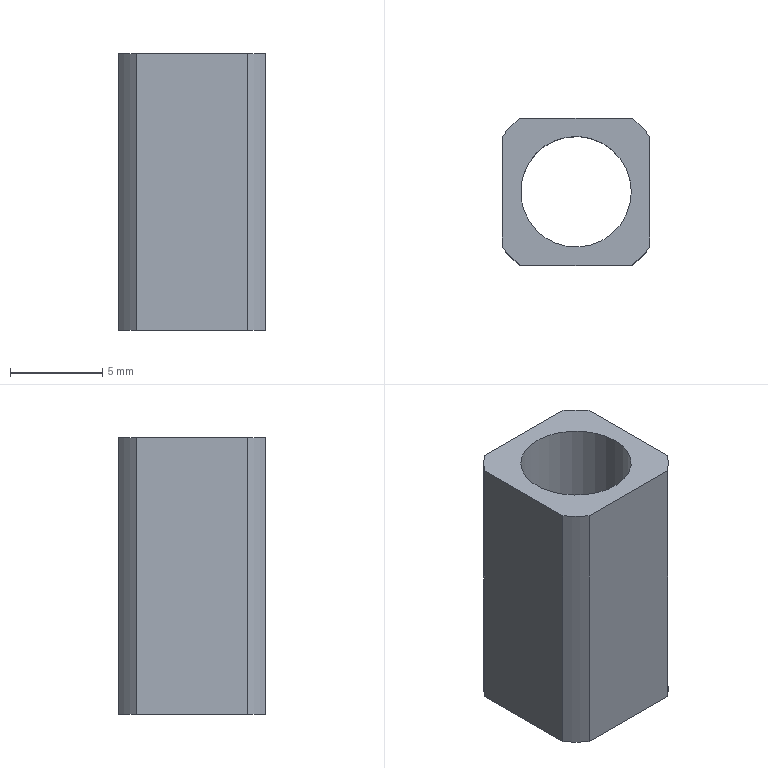NC program | NX | posted with a generic post | part box 8 x 8 x 15 mm
Whole program:
N10 G17 G21 G94 G90
(PLANAR_MILL , TOOL : D8开粗)
N12 T01 M6
N14 G53
N16 G17 G0 G90 X15.25 Y0. S2000 M3
N18 G43 Z10.05 H1
N20 Z2.05
N22 G94 G1 Z0.05 F800.
N24 X5.25
N26 G2 X0. Y-5.25 R5.25
N28 X5.25 Y0. R-5.25
N30 G1 X15.25
N32 Z2.05
N34 G0 Z10.05
(ADAPTIVE_MILLING , TOOL : D8开粗)
N36 Z10.15 S3000
N38 X-17.042 Y-1.094
N40 Z-13.
N42 G1 X-16.892 Y-1.097 Z-13.937 F1000.
N44 X-16.742 Y-1.099 Z-14.308
N46 X-16.592 Y-1.102 Z-14.58
N48 X-16.442 Y-1.105 Z-14.8
N50 X-16.292 Y-1.107 Z-14.984
N52 X-16.142 Y-1.11 Z-15.142
N54 X-15.992 Y-1.113 Z-15.28
N56 X-15.842 Y-1.115 Z-15.4
N58 X-15.692 Y-1.118 Z-15.505
N60 X-15.542 Y-1.121 Z-15.598
N62 X-15.392 Y-1.123 Z-15.679
N64 X-15.242 Y-1.126 Z-15.75
N66 X-15.092 Y-1.129 Z-15.81
N68 X-14.942 Y-1.131 Z-15.862
N70 X-14.792 Y-1.134 Z-15.905
N72 X-14.642 Y-1.137 Z-15.939
N74 X-14.492 Y-1.139 Z-15.966
N76 X-14.342 Y-1.142 Z-15.985
N78 X-14.192 Y-1.145 Z-15.996
N80 X-14.043 Y-1.147 Z-16.
N82 X-12.799 Y-1.169
N84 G3 X-12.014 Y-0.604 R0.808
N86 X-11.826 Y1.614 R11.177
N88 G1 X-11.782 Y7.095
N90 G2 X-9.344 Y10.662 R4.681
N92 X-5.735 Y11.668 R8.663
N94 X0.162 Y11.795 R77.314
N96 X7.156 Y11.776 R258.292
N98 X10.72 Y9.242 R4.72
N100 X11.678 Y5.618 R8.934
N102 X11.795 Y-0.155 R82.543
N104 X11.776 Y-7.161 R292.319
N106 X9.265 Y-10.715 R4.695
N108 X5.52 Y-11.688 R9.057
N110 X-0.703 Y-11.796 R97.121
N112 X-7.161 Y-11.776 R245.126
N114 X-10.715 Y-9.265 R4.696
N116 X-11.675 Y-5.669 R8.872
N118 X-11.668 Y0.672 R45.823
N120 G3 X-11.577 Y6.026 R963.899
N122 G2 X-8.439 Y10.473 R5.565
N124 X-4.388 Y11.473 R10.591
N126 X1.635 Y11.595 R90.551
N128 X6.093 Y11.568 R96.361
N130 X10.489 Y8.407 R5.576
N132 X11.474 Y4.376 R10.641
N134 X11.595 Y-2.221 R100.16
N136 X11.565 Y-6.136 R71.688
N138 X8.395 Y-10.499 R5.568
N140 X4.413 Y-11.472 R10.62
N142 X-2.21 Y-11.595 R98.687
N144 X-6.136 Y-11.565 R71.79
N146 X-10.506 Y-8.382 R5.572
N148 X-11.475 Y-4.372 R10.694
N150 X-11.47 Y0.664 R42.379
N152 X-11.374 Y5.194 R380.588
N154 X-7.691 Y10.298 R6.176
N156 X-3.525 Y11.263 R11.89
N158 X2.822 Y11.395 R94.709
N160 X5.618 Y11.316 R21.328
N162 X10.315 Y7.652 R6.193
N164 X11.274 Y3.383 R12.149
N166 X11.395 Y-3.015 R104.262
N168 X11.315 Y-5.636 R19.37
N170 X7.658 Y-10.315 R6.184
N172 X3.463 Y-11.269 R12.036
N174 X-3.41 Y-11.395 R107.036
N176 X-5.976 Y-11.254 R12.481
N178 X-10.341 Y-7.6 R6.222
N180 X-11.279 Y-3.175 R12.209
N182 X-11.231 Y2.429 R98.325
N184 X-11.072 Y5.231 R16.901
N186 X-7.005 Y10.134 R6.683
N188 X-2.5 Y11.077 R13.524
N190 X4.521 Y11.154 R76.078
N192 X10.106 Y7.062 R6.639
N194 X11.066 Y2.663 R13.127
N196 X11.16 Y-4.459 R82.201
N198 X7.056 Y-10.111 R6.636
N200 X2.704 Y-11.063 R13.088
N202 X-4.493 Y-11.157 R78.628
N204 X-10.077 Y-7.131 R6.62
N206 X-11.045 Y-2.484 R12.49
N208 X-10.968 Y3.923 R83.072
N210 X-6.541 Y9.897 R7.057
N212 X-1.963 Y10.863 R14.094
N214 X3.884 Y10.945 R54.17
N216 X9.887 Y6.556 R7.016
N218 X10.85 Y2.13 R13.757
N220 X10.941 Y-3.941 R51.906
N222 X6.521 Y-9.904 R7.018
N224 X1.916 Y-10.866 R14.175
N226 X-3.955 Y-10.939 R51.457
N228 X-9.91 Y-6.504 R7.014
N230 X-10.814 Y-1.867 R13.325
N232 X-10.752 Y3.505 R47.883
N234 X-6.022 Y9.702 R7.399
N236 X-1.339 Y10.659 R14.972
N238 X3.507 Y10.713 R34.845
N240 X9.627 Y6.189 R7.308
N242 X10.643 Y1.546 R14.275
N244 X10.717 Y-3.474 R35.968
N246 X6.142 Y-9.648 R7.315
N248 X1.595 Y-10.64 R14.298
N250 X-3.475 Y-10.717 R35.976
N252 X-9.664 Y-6.092 R7.298
N254 X-10.585 Y-1.355 R13.912
N256 X-10.519 Y3.215 R30.019
N258 X-5.678 Y9.448 R7.656
N260 X-0.901 Y10.446 R15.28
N262 X3.293 Y10.459 R22.898
N264 X9.397 Y5.783 R7.559
N266 X10.44 Y0.967 R14.889
N268 X10.458 Y-3.302 R23.023
N270 X5.812 Y-9.386 R7.548
N272 X1.021 Y-10.436 R14.775
N274 X-3.297 Y-10.459 R23.268
N276 X-9.469 Y-5.58 R7.546
N278 X-10.365 Y-0.785 R14.819
N280 X-10.204 Y3.377 R17.96
N282 X-5.345 Y9.2 R7.864
N284 X-0.475 Y10.234 R15.571
N286 X3.584 Y10.106 R14.623
N288 X9.134 Y5.477 R7.754
N290 X10.228 Y0.544 R15.103
N292 X10.126 Y-3.492 R15.05
N294 X5.435 Y-9.154 R7.756
N296 X0.525 Y-10.23 R15.218
N298 X-3.511 Y-10.122 R14.971
N300 X-9.214 Y-5.24 R7.724
N302 X-10.144 Y-0.3 R15.2
N304 X-9.73 Y3.957 R12.121
N306 X-4.905 Y9.005 R8.107
N308 X0.644 Y10.054 R16.429
N310 X5.363 Y9.083 R9.1
N312 X9.18 Y4.424 R8.361
N314 X9.955 Y-2.677 R16.603
N316 X5.153 Y-8.889 R7.914
N318 X0.025 Y-10.02 R15.271
N320 X-4.364 Y-9.534 R10.49
N322 X-9.041 Y-4.711 R7.991
N324 X-9.733 Y2.631 R14.976
N326 X-4.844 Y8.656 R8.163
N328 X2.526 Y9.667 R14.2
N330 X8.644 Y4.84 R8.042
N332 X9.668 Y-2.525 R14.119
N334 X4.901 Y-8.617 R8.024
N336 X-2.509 Y-9.67 R14.119
N338 X-8.649 Y-4.746 R7.958
N340 X-9.446 Y2.464 R13.067
N342 X-4.563 Y8.406 R8.261
N344 X2.353 Y9.372 R12.559
N346 X8.375 Y4.592 R8.12
N348 X9.369 Y-2.369 R12.455
N350 X4.633 Y-8.357 R8.107
N352 X-2.325 Y-9.376 R12.477
N354 X-8.366 Y-4.514 R8.022
N356 X-9.112 Y2.46 R11.549
N358 X-4.31 Y8.146 R8.33
N360 X2.181 Y9.065 R11.251
N362 X8.076 Y4.414 R8.149
N364 X9.054 Y-2.235 R11.133
N366 X4.337 Y-8.113 R8.16
N368 X-2.294 Y-9.041 R11.08
N370 X-8.088 Y-4.277 R8.055
N372 X-8.762 Y2.442 R10.379
N374 X-7.774 Y4.726 R8.558
N376 G1 X-7.319 Y5.491
N378 G2 X-5.489 Y7.321 R10.635
N380 X-3.39 Y8.269 R7.25
N382 X1.932 Y8.765 R10.975
N384 X4.417 Y7.877 R8.348
N386 G1 X4.726 Y7.774
N388 X5.491 Y7.319
N390 G2 X7.321 Y5.489 R10.635
N392 X8.236 Y3.47 R6.929
N394 X8.791 Y-1.775 R11.171
N396 X7.879 Y-4.41 R8.25
N398 G1 X7.774 Y-4.726
N400 X7.319 Y-5.491
N402 G2 X5.489 Y-7.321 R10.635
N404 X3.469 Y-8.237 R6.939
N406 X-1.703 Y-8.8 R11.199
N408 X-4.365 Y-7.894 R8.205
N410 G1 X-4.726 Y-7.774
N412 X-5.491 Y-7.319
N414 G2 X-7.321 Y-5.489 R10.635
N416 X-8.055 Y-3.883 R4.818
N418 X-8.648 Y1.286 R11.376
N420 X-8.116 Y3.313 R12.901
N422 G1 X-8.055 Y3.883
N424 G2 X-7.319 Y5.491 R4.82
N426 X-5.489 Y7.321 R10.635
N428 X-3.385 Y8.155 R4.891
N430 X0.551 Y8.602 R14.975
N432 X2.98 Y8.15 R11.554
N434 G1 X3.883 Y8.055
N436 X4.429 Y7.873
N438 G3 X5.384 Y9.015 R0.8
N440 X5.034 Y9.367 Z-15.969 R1.074
N442 G1 X4.158 Y10.019 Z-15.9
N444 X3.084 Y10.819 F10000.
N446 G3 X2.637 Y10.977 R0.812
N448 G1 X-2.091 Y11.159
N450 G3 X-2.628 Y10.979 R0.806
N452 G1 X-3.724 Y10.084
N454 X-4.52 Y9.427 Z-15.965 F1000.
N456 G3 X-4.764 Y8.936 Z-16. R0.802
N458 X-3.883 Y8.055 R0.8
N460 G2 X-0.226 Y8.349 R35.084
N462 X1.762 Y8.15 R14.752
N464 G1 X2.987
N466 G3 X3.787 Y8.945 R0.8
N468 X3.444 Y9.61 Z-15.951 R0.83
N470 G1 X2.82 Y10.135 Z-15.9
N472 X1.709 Y11.067 F10000.
N474 G3 X1.195 Y11.254 R0.807
N476 G1 X-1.207
N478 G3 X-1.721 Y11.067 R0.807
N480 G1 X-2.812 Y10.151
N482 X-3.561 Y9.515 Z-15.962 F1000.
N484 G3 X-3.799 Y8.97 Z-16. R0.8
N486 X-2.999 Y8.15 R0.8
N488 G1 X3.001
N490 G2 X4.726 Y7.774 R4.82
N492 G1 X5.491 Y7.319
N494 G2 X7.321 Y5.489 R10.635
N496 X8.169 Y3.304 R4.943
N498 X8.59 Y-0.702 R14.448
N500 X8.15 Y-2.979 R12.224
N502 G1 X8.055 Y-3.883
N504 X7.873 Y-4.429
N506 G3 X9.015 Y-5.384 R0.8
N508 X9.367 Y-5.034 Z-15.969 R1.074
N510 G1 X10.019 Y-4.158 Z-15.9
N512 X10.819 Y-3.084 F10000.
N514 G3 X10.977 Y-2.637 R0.812
N516 G1 X11.159 Y2.091
N518 G3 X10.979 Y2.628 R0.806
N520 G1 X10.084 Y3.724
N522 X9.427 Y4.52 Z-15.965 F1000.
N524 G3 X8.936 Y4.764 Z-16. R0.802
N526 X8.055 Y3.883 R0.8
N528 G2 X8.346 Y0.184 R34.384
N530 X8.15 Y-1.754 R15.228
N532 G1 Y-3.001
N534 G3 X8.945 Y-3.801 R0.8
N536 X9.61 Y-3.458 Z-15.951 R0.83
N538 G1 X10.135 Y-2.833 Z-15.9
N540 X11.067 Y-1.723 F10000.
N542 G3 X11.254 Y-1.209 R0.807
N544 G1 Y1.207
N546 G3 X11.067 Y1.721 R0.807
N548 G1 X10.151 Y2.812
N550 X9.515 Y3.561 Z-15.962 F1000.
N552 G3 X8.97 Y3.799 Z-16. R0.8
N554 X8.15 Y2.999 R0.8
N556 G1 Y-3.001
N558 G2 X7.774 Y-4.726 R4.82
N560 G1 X7.319 Y-5.491
N562 G2 X5.489 Y-7.321 R10.635
N564 X3.304 Y-8.169 R4.943
N566 X-0.677 Y-8.59 R14.447
N568 X-2.955 Y-8.152 R11.964
N570 G1 X-3.883 Y-8.055
N572 X-4.381 Y-7.889
N574 G3 X-5.345 Y-9.015 R0.8
N576 X-4.989 Y-9.381 Z-15.968 R1.048
N578 G1 X-4.126 Y-10.024 Z-15.9
N580 X-3.039 Y-10.835 F10000.
N582 G3 X-2.589 Y-10.993 R0.812
N584 G1 X2.091 Y-11.159
N586 G3 X2.625 Y-10.979 R0.806
N588 G1 X3.722 Y-10.084
N590 X4.52 Y-9.427 Z-15.965 F1000.
N592 G3 X4.764 Y-8.937 Z-16. R0.802
N594 X3.883 Y-8.055 R0.8
N596 G2 X0.134 Y-8.344 R33.059
N598 X-1.73 Y-8.15 R15.834
N600 G1 X-3.001
N602 G3 X-3.801 Y-8.945 R0.8
N604 X-3.458 Y-9.61 Z-15.951 R0.83
N606 G1 X-2.833 Y-10.135 Z-15.9
N608 X-1.723 Y-11.067 F10000.
N610 G3 X-1.209 Y-11.254 R0.807
N612 G1 X1.207
N614 G3 X1.721 Y-11.067 R0.807
N616 G1 X2.812 Y-10.151
N618 X3.561 Y-9.515 Z-15.962 F1000.
N620 G3 X3.799 Y-8.97 Z-16. R0.8
N622 X2.999 Y-8.15 R0.8
N624 G1 X-3.001
N626 G2 X-4.726 Y-7.774 R4.82
N628 G1 X-5.491 Y-7.319
N630 G2 X-7.321 Y-5.489 R10.635
N632 X-8.055 Y-3.883 R4.818
N634 X-8.433 Y-1.021 R51.208
N636 X-8.15 Y2.209 R11.845
N638 X-8.115 Y3.324 R8.238
N640 G3 X-8.973 Y4.207 R0.8
N642 X-9.582 Y3.851 Z-15.954 R0.842
N644 G1 X-10.125 Y3.179 Z-15.9
N646 X-11.042 Y2.043 F10000.
N648 G3 X-11.219 Y1.532 R0.807
N650 G1 X-11.183 Y-1.868
N652 G3 X-11.008 Y-2.359 R0.808
N654 G1 X-10.11 Y-3.481
N656 X-9.457 Y-4.29 Z-15.965 F1000.
N658 G3 X-8.976 Y-4.539 Z-16. R0.802
N660 X-8.079 Y-3.66 R0.8
N662 G2 X-8.15 Y0.431 R23.135
N664 G1 Y2.231
N666 G3 X-9.03 Y3.111 R0.88
N668 X-9.91 Y2.231 R0.88
N670 G1 Y-2.825
N672 G3 X-9.03 Y-3.705 R0.88
N674 X-8.15 Y-2.825 R0.88
N676 G1 Y0.45
N678 G3 X-9.038 Y1.254 R0.808
N680 G1 X-10.141 Y1.144
N682 X-10.29 Y1.129 Z-15.996
N684 X-10.44 Y1.114 Z-15.985
N686 X-10.589 Y1.099 Z-15.966
N688 X-10.738 Y1.084 Z-15.939
N690 X-10.887 Y1.069 Z-15.905
N692 X-11.037 Y1.054 Z-15.862
N694 X-11.186 Y1.039 Z-15.81
N696 X-11.335 Y1.024 Z-15.75
N698 X-11.484 Y1.009 Z-15.679
N700 X-11.634 Y0.995 Z-15.598
N702 X-11.783 Y0.98 Z-15.505
N704 X-11.932 Y0.965 Z-15.4
N706 X-12.081 Y0.95 Z-15.28
N708 X-12.231 Y0.935 Z-15.142
N710 X-12.38 Y0.92 Z-14.984
N712 X-12.529 Y0.905 Z-14.8
N714 X-12.678 Y0.89 Z-14.58
N716 X-12.828 Y0.875 Z-14.308
N718 X-12.977 Y0.86 Z-13.937
N720 X-13.126 Y0.845 Z-13.
N722 G0 Z10.15
N724 M5
(DRILLING , TOOL : D10点钻)
N726 T03 M6
N728 G53
N730 G17 G0 G90 X0. Y0. S1200 M3
N732 G43 Z22.5 H3
N734 G94 G81 G99 Z-1.5 F100. R3.
N736 G80
N738 G0 X0. Y0. Z22.5
N740 M5
(DRILLING_1 , TOOL : 5.1钻头)
N742 T04 M6
N744 G53
N746 G17 G0 G90 X0. Y0. S1600 M3
N748 G43 Z22.5 H4
N750 G94 G83 G99 Z-28. F150. Q2. R3.
N752 G80
N754 G0 X0. Y0. Z22.5
N756 M5
(DRILLING_COPY , TOOL : D10点钻)
N758 T03 M6
N760 G53
N762 G17 G0 G90 X0. Y0. S1600 M3
N764 G43 Z22.5 H3
N766 G94 G81 G99 Z-3. F150. R3.
N768 G80
N770 G0 X0. Y0. Z22.5
N772 M5
(PLANAR_MILL_1 , TOOL : D4)
N774 T07 M6
N776 G53
N778 G17 G0 G90 X0.206 Y-0.165 S3000 M3
N780 G43 Z10. H7
N782 Z-7.
N784 G94 G1 Z-9. F300.
N786 G41 X0.403 Y-0.2 D7
N788 X0.55
N790 G3 X0.75 Y0. R0.2
N792 X0. Y0.75 R0.75
N794 X0.75 Y0. R-0.75
N796 X0.55 Y0.2 R0.2
N798 G40
N800 G1 X0.353 Y0.165
N802 X0.453 Y-0.165
N804 G41 X0.65 Y-0.2
N806 G3 X0.85 Y0. R0.2
N808 X0. Y0.85 R0.85
N810 X0.85 Y0. R-0.85
N812 X0.65 Y0.2 R0.2
N814 G40
N816 G1 X0.453 Y0.165
N818 X0.553 Y-0.165
N820 G41 X0.75 Y-0.2
N822 G3 X0.95 Y0. R0.2
N824 X0. Y0.95 R0.95
N826 X0.95 Y0. R-0.95
N828 X0.75 Y0.2 R0.2
N830 G40
N832 G1 X0.553 Y0.165
N834 X0.653 Y-0.165
N836 G41 X0.85 Y-0.2
N838 G3 X1.05 Y0. R0.2
N840 X0. Y1.05 R1.05
N842 X1.05 Y0. R-1.05
N844 X0.85 Y0.2 R0.2
N846 G40
N848 G1 X0.653 Y0.165
N850 X0.753 Y-0.165
N852 G41 X0.95 Y-0.2
N854 G3 X1.15 Y0. R0.2
N856 X0. Y1.15 R1.15
N858 X1.15 Y0. R-1.15
N860 X0.95 Y0.2 R0.2
N862 G40
N864 G1 X0.753 Y0.165
N866 X0.853 Y-0.165
N868 G41 X1.05 Y-0.2
N870 G3 X1.25 Y0. R0.2
N872 X0. Y1.25 R1.25
N874 X1.25 Y0. R-1.25
N876 X1.05 Y0.2 R0.2
N878 G1 X0.929
N880 G40
N882 X0.732 Y0.165
N884 Z-7.
N886 G0 Z10.
N888 M5
(PLANAR_MILL_3_COPY_1 , TOOL : D6倒角刀)
N890 T05 M6
N892 G53
N894 G17 G0 G90 X-8. Y0. S3000 M3
N896 G43 Z10. H5
N898 Z0.
N900 G94 G1 Z-2. F800.
N902 X-6.
N904 Y3.
N906 G2 X-5.6 Y4.2 R2.
N908 X-4.2 Y5.6 R7.
N910 X-3. Y6. R2.
N912 G1 X3.
N914 G2 X4.2 Y5.6 R2.
N916 X5.6 Y4.2 R7.
N918 X6. Y3. R2.
N920 G1 Y-3.
N922 G2 X5.6 Y-4.2 R2.
N924 X4.2 Y-5.6 R7.
N926 X3. Y-6. R2.
N928 G1 X-3.
N930 G2 X-4.2 Y-5.6 R2.
N932 X-5.6 Y-4.2 R7.
N934 X-6. Y-3. R2.
N936 G1 Y0.
N938 X-8.
N940 Z0.
N942 G0 Z10.
N944 M5
(PLANAR_MILL_COPY_COPY , TOOL : D8精光)
N946 T02 M6
N948 G53
N950 G17 G0 G90 X8.25 Y0. S3000 M3
N952 G43 Z10. H2
N954 Z2.
N956 G94 G1 Z0. F600.
N958 X5.25
N960 G2 X0. Y-5.25 R5.25
N962 X5.25 Y0. R-5.25
N964 G1 X8.25
N966 Z2.
N968 G0 Z10.
(PLANAR_MILL_1_COPY , TOOL : D8精光)
N970 X-1.174 Y-10.985
N972 Z10.
N974 Z-14.
N976 G1 Z-16.
N978 G41 X-1. Y-10. D2
N980 G3 X-3. Y-8. R2.
N982 G2 X-5.4 Y-7.2 R4.
N984 X-7.2 Y-5.4 R9.
N986 X-8. Y-3. R4.
N988 G1 Y3.
N990 G2 X-7.2 Y5.4 R4.
N992 X-5.4 Y7.2 R9.
N994 X-3. Y8. R4.
N996 G1 X3.
N998 G2 X5.4 Y7.2 R4.
N1000 X7.2 Y5.4 R9.
N1002 X8. Y3. R4.
N1004 G1 Y-3.
N1006 G2 X7.2 Y-5.4 R4.
N1008 X5.4 Y-7.2 R9.
N1010 X3. Y-8. R4.
N1012 G1 X-3.
N1014 G3 X-5. Y-10. R2.
N1016 G40
N1018 G1 X-4.826 Y-10.985
N1020 X-1.174
N1022 G41 X-1. Y-10.
N1024 G3 X-3. Y-8. R2.
N1026 G2 X-5.4 Y-7.2 R4.
N1028 X-7.2 Y-5.4 R9.
N1030 X-8. Y-3. R4.
N1032 G1 Y3.
N1034 G2 X-7.2 Y5.4 R4.
N1036 X-5.4 Y7.2 R9.
N1038 X-3. Y8. R4.
N1040 G1 X3.
N1042 G2 X5.4 Y7.2 R4.
N1044 X7.2 Y5.4 R9.
N1046 X8. Y3. R4.
N1048 G1 Y-3.
N1050 G2 X7.2 Y-5.4 R4.
N1052 X5.4 Y-7.2 R9.
N1054 X3. Y-8. R4.
N1056 G1 X-3.
N1058 G3 X-5. Y-10. R2.
N1060 G40
N1062 G1 X-4.826 Y-10.985
N1064 Z-14.
N1066 G0 Z10.
N1068 M5
N1070 M2